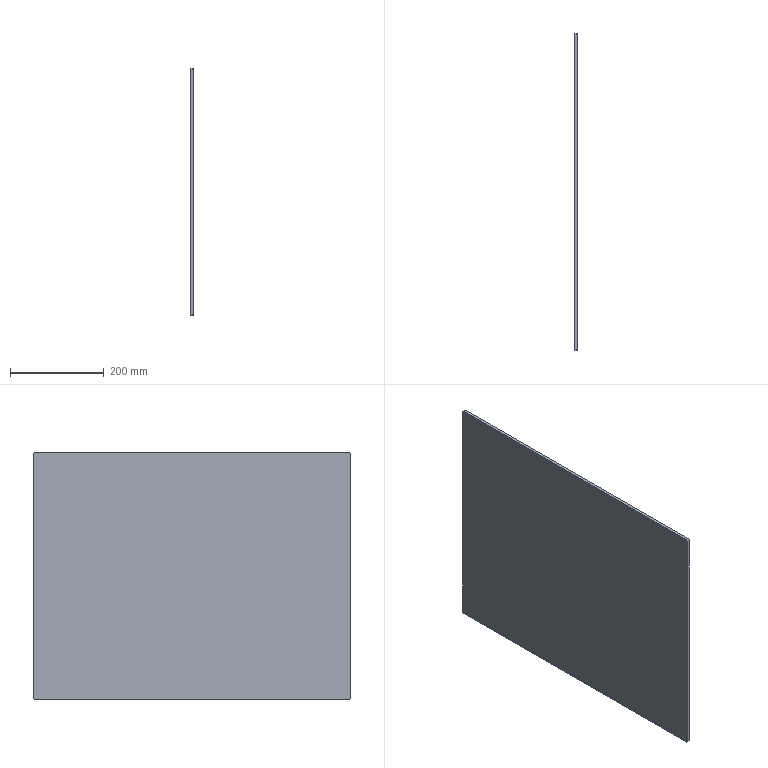Part | SolidWorks | features Chamfer 1, Extrusion 1 | 1 solid | 10 faces | box 6 x 677 x 528 mm | volume 2144688 mm3 | plane 10
STEP:
#1=CARTESIAN_POINT('',(3.,-336.5,-264.));
#2=VERTEX_POINT('',#1);
#3=CARTESIAN_POINT('',(3.,336.5,-264.));
#4=VERTEX_POINT('',#3);
#5=CARTESIAN_POINT('',(3.,338.5,-264.));
#6=DIRECTION('',(0.,1.,0.));
#7=VECTOR('',#6,1000.);
#8=LINE('',#5,#7);
#9=EDGE_CURVE('',#2,#4,#8,.T.);
#10=ORIENTED_EDGE('',*,*,#9,.F.);
#11=CARTESIAN_POINT('',(-3.,-336.5,-264.));
#12=VERTEX_POINT('',#11);
#13=CARTESIAN_POINT('',(3.,-336.5,-264.));
#14=DIRECTION('',(-1.,0.,0.));
#15=VECTOR('',#14,1000.);
#16=LINE('',#13,#15);
#17=EDGE_CURVE('',#2,#12,#16,.T.);
#18=ORIENTED_EDGE('',*,*,#17,.T.);
#19=CARTESIAN_POINT('',(-3.,336.5,-264.));
#20=VERTEX_POINT('',#19);
#21=CARTESIAN_POINT('',(-3.,338.5,-264.));
#22=DIRECTION('',(0.,1.,0.));
#23=VECTOR('',#22,1000.);
#24=LINE('',#21,#23);
#25=EDGE_CURVE('',#12,#20,#24,.T.);
#26=ORIENTED_EDGE('',*,*,#25,.T.);
#27=CARTESIAN_POINT('',(3.,336.5,-264.));
#28=DIRECTION('',(1.,0.,0.));
#29=VECTOR('',#28,1000.);
#30=LINE('',#27,#29);
#31=EDGE_CURVE('',#20,#4,#30,.T.);
#32=ORIENTED_EDGE('',*,*,#31,.T.);
#33=EDGE_LOOP('',(#10,#18,#26,#32));
#34=FACE_OUTER_BOUND('',#33,.T.);
#35=CARTESIAN_POINT('',(3.,338.5,-264.));
#36=DIRECTION('',(0.,0.,1.));
#37=DIRECTION('',(0.,-1.,0.));
#38=AXIS2_PLACEMENT_3D('',#35,#36,#37);
#39=PLANE('',#38);
#40=ADVANCED_FACE('',(#34),#39,.F.);
#41=CARTESIAN_POINT('',(3.,338.5,-262.));
#42=VERTEX_POINT('',#41);
#43=CARTESIAN_POINT('',(3.,338.5,262.));
#44=VERTEX_POINT('',#43);
#45=CARTESIAN_POINT('',(3.,338.5,264.));
#46=DIRECTION('',(0.,0.,1.));
#47=VECTOR('',#46,1000.);
#48=LINE('',#45,#47);
#49=EDGE_CURVE('',#42,#44,#48,.T.);
#50=ORIENTED_EDGE('',*,*,#49,.F.);
#51=CARTESIAN_POINT('',(-3.,338.5,-262.));
#52=VERTEX_POINT('',#51);
#53=CARTESIAN_POINT('',(3.,338.5,-262.));
#54=DIRECTION('',(-1.,0.,0.));
#55=VECTOR('',#54,1000.);
#56=LINE('',#53,#55);
#57=EDGE_CURVE('',#42,#52,#56,.T.);
#58=ORIENTED_EDGE('',*,*,#57,.T.);
#59=CARTESIAN_POINT('',(-3.,338.5,262.));
#60=VERTEX_POINT('',#59);
#61=CARTESIAN_POINT('',(-3.,338.5,264.));
#62=DIRECTION('',(0.,0.,1.));
#63=VECTOR('',#62,1000.);
#64=LINE('',#61,#63);
#65=EDGE_CURVE('',#52,#60,#64,.T.);
#66=ORIENTED_EDGE('',*,*,#65,.T.);
#67=CARTESIAN_POINT('',(3.,338.5,262.));
#68=DIRECTION('',(1.,0.,0.));
#69=VECTOR('',#68,1000.);
#70=LINE('',#67,#69);
#71=EDGE_CURVE('',#60,#44,#70,.T.);
#72=ORIENTED_EDGE('',*,*,#71,.T.);
#73=EDGE_LOOP('',(#50,#58,#66,#72));
#74=FACE_OUTER_BOUND('',#73,.T.);
#75=CARTESIAN_POINT('',(3.,338.5,264.));
#76=DIRECTION('',(0.,-1.,0.));
#77=DIRECTION('',(0.,0.,-1.));
#78=AXIS2_PLACEMENT_3D('',#75,#76,#77);
#79=PLANE('',#78);
#80=ADVANCED_FACE('',(#74),#79,.F.);
#81=CARTESIAN_POINT('',(-3.,336.5,264.));
#82=VERTEX_POINT('',#81);
#83=CARTESIAN_POINT('',(-3.,-336.5,264.));
#84=VERTEX_POINT('',#83);
#85=CARTESIAN_POINT('',(-3.,338.5,264.));
#86=DIRECTION('',(0.,-1.,0.));
#87=VECTOR('',#86,1000.);
#88=LINE('',#85,#87);
#89=EDGE_CURVE('',#82,#84,#88,.T.);
#90=ORIENTED_EDGE('',*,*,#89,.T.);
#91=CARTESIAN_POINT('',(3.,-336.5,264.));
#92=VERTEX_POINT('',#91);
#93=CARTESIAN_POINT('',(3.,-336.5,264.));
#94=DIRECTION('',(1.,0.,0.));
#95=VECTOR('',#94,1000.);
#96=LINE('',#93,#95);
#97=EDGE_CURVE('',#84,#92,#96,.T.);
#98=ORIENTED_EDGE('',*,*,#97,.T.);
#99=CARTESIAN_POINT('',(3.,336.5,264.));
#100=VERTEX_POINT('',#99);
#101=CARTESIAN_POINT('',(3.,338.5,264.));
#102=DIRECTION('',(0.,-1.,0.));
#103=VECTOR('',#102,1000.);
#104=LINE('',#101,#103);
#105=EDGE_CURVE('',#100,#92,#104,.T.);
#106=ORIENTED_EDGE('',*,*,#105,.F.);
#107=CARTESIAN_POINT('',(3.,336.5,264.));
#108=DIRECTION('',(-1.,0.,0.));
#109=VECTOR('',#108,1000.);
#110=LINE('',#107,#109);
#111=EDGE_CURVE('',#100,#82,#110,.T.);
#112=ORIENTED_EDGE('',*,*,#111,.T.);
#113=EDGE_LOOP('',(#90,#98,#106,#112));
#114=FACE_OUTER_BOUND('',#113,.T.);
#115=CARTESIAN_POINT('',(3.,338.5,264.));
#116=DIRECTION('',(0.,0.,-1.));
#117=DIRECTION('',(0.,1.,0.));
#118=AXIS2_PLACEMENT_3D('',#115,#116,#117);
#119=PLANE('',#118);
#120=ADVANCED_FACE('',(#114),#119,.F.);
#121=CARTESIAN_POINT('',(3.,-338.5,262.));
#122=VERTEX_POINT('',#121);
#123=CARTESIAN_POINT('',(3.,-338.5,-262.));
#124=VERTEX_POINT('',#123);
#125=CARTESIAN_POINT('',(3.,-338.5,264.));
#126=DIRECTION('',(0.,0.,-1.));
#127=VECTOR('',#126,1000.);
#128=LINE('',#125,#127);
#129=EDGE_CURVE('',#122,#124,#128,.T.);
#130=ORIENTED_EDGE('',*,*,#129,.F.);
#131=CARTESIAN_POINT('',(-3.,-338.5,262.));
#132=VERTEX_POINT('',#131);
#133=CARTESIAN_POINT('',(3.,-338.5,262.));
#134=DIRECTION('',(-1.,0.,0.));
#135=VECTOR('',#134,1000.);
#136=LINE('',#133,#135);
#137=EDGE_CURVE('',#122,#132,#136,.T.);
#138=ORIENTED_EDGE('',*,*,#137,.T.);
#139=CARTESIAN_POINT('',(-3.,-338.5,-262.));
#140=VERTEX_POINT('',#139);
#141=CARTESIAN_POINT('',(-3.,-338.5,264.));
#142=DIRECTION('',(0.,0.,-1.));
#143=VECTOR('',#142,1000.);
#144=LINE('',#141,#143);
#145=EDGE_CURVE('',#132,#140,#144,.T.);
#146=ORIENTED_EDGE('',*,*,#145,.T.);
#147=CARTESIAN_POINT('',(3.,-338.5,-262.));
#148=DIRECTION('',(1.,0.,0.));
#149=VECTOR('',#148,1000.);
#150=LINE('',#147,#149);
#151=EDGE_CURVE('',#140,#124,#150,.T.);
#152=ORIENTED_EDGE('',*,*,#151,.T.);
#153=EDGE_LOOP('',(#130,#138,#146,#152));
#154=FACE_OUTER_BOUND('',#153,.T.);
#155=CARTESIAN_POINT('',(3.,-338.5,264.));
#156=DIRECTION('',(0.,1.,0.));
#157=DIRECTION('',(0.,0.,1.));
#158=AXIS2_PLACEMENT_3D('',#155,#156,#157);
#159=PLANE('',#158);
#160=ADVANCED_FACE('',(#154),#159,.F.);
#161=ORIENTED_EDGE('',*,*,#105,.T.);
#162=CARTESIAN_POINT('',(3.,-300.25,300.25));
#163=DIRECTION('',(0.,-0.7071,-0.7071));
#164=VECTOR('',#163,1000.);
#165=LINE('',#162,#164);
#166=EDGE_CURVE('',#92,#122,#165,.T.);
#167=ORIENTED_EDGE('',*,*,#166,.T.);
#168=ORIENTED_EDGE('',*,*,#129,.T.);
#169=CARTESIAN_POINT('',(3.,-300.25,-300.25));
#170=DIRECTION('',(0.,0.7071,-0.7071));
#171=VECTOR('',#170,1000.);
#172=LINE('',#169,#171);
#173=EDGE_CURVE('',#124,#2,#172,.T.);
#174=ORIENTED_EDGE('',*,*,#173,.T.);
#175=ORIENTED_EDGE('',*,*,#9,.T.);
#176=CARTESIAN_POINT('',(3.,300.25,-300.25));
#177=DIRECTION('',(0.,0.7071,0.7071));
#178=VECTOR('',#177,1000.);
#179=LINE('',#176,#178);
#180=EDGE_CURVE('',#4,#42,#179,.T.);
#181=ORIENTED_EDGE('',*,*,#180,.T.);
#182=ORIENTED_EDGE('',*,*,#49,.T.);
#183=CARTESIAN_POINT('',(3.,300.25,300.25));
#184=DIRECTION('',(0.,-0.7071,0.7071));
#185=VECTOR('',#184,1000.);
#186=LINE('',#183,#185);
#187=EDGE_CURVE('',#44,#100,#186,.T.);
#188=ORIENTED_EDGE('',*,*,#187,.T.);
#189=EDGE_LOOP('',(#161,#167,#168,#174,#175,#181,#182,#188));
#190=FACE_OUTER_BOUND('',#189,.T.);
#191=CARTESIAN_POINT('',(3.,0.,0.));
#192=DIRECTION('',(1.,0.,0.));
#193=DIRECTION('',(0.,0.,-1.));
#194=AXIS2_PLACEMENT_3D('',#191,#192,#193);
#195=PLANE('',#194);
#196=ADVANCED_FACE('',(#190),#195,.T.);
#197=ORIENTED_EDGE('',*,*,#145,.F.);
#198=CARTESIAN_POINT('',(-3.,-338.5,262.));
#199=DIRECTION('',(0.,0.7071,0.7071));
#200=VECTOR('',#199,1000.);
#201=LINE('',#198,#200);
#202=EDGE_CURVE('',#132,#84,#201,.T.);
#203=ORIENTED_EDGE('',*,*,#202,.T.);
#204=ORIENTED_EDGE('',*,*,#89,.F.);
#205=CARTESIAN_POINT('',(-3.,336.5,264.));
#206=DIRECTION('',(0.,0.7071,-0.7071));
#207=VECTOR('',#206,1000.);
#208=LINE('',#205,#207);
#209=EDGE_CURVE('',#82,#60,#208,.T.);
#210=ORIENTED_EDGE('',*,*,#209,.T.);
#211=ORIENTED_EDGE('',*,*,#65,.F.);
#212=CARTESIAN_POINT('',(-3.,338.5,-262.));
#213=DIRECTION('',(0.,-0.7071,-0.7071));
#214=VECTOR('',#213,1000.);
#215=LINE('',#212,#214);
#216=EDGE_CURVE('',#52,#20,#215,.T.);
#217=ORIENTED_EDGE('',*,*,#216,.T.);
#218=ORIENTED_EDGE('',*,*,#25,.F.);
#219=CARTESIAN_POINT('',(-3.,-336.5,-264.));
#220=DIRECTION('',(0.,-0.7071,0.7071));
#221=VECTOR('',#220,1000.);
#222=LINE('',#219,#221);
#223=EDGE_CURVE('',#12,#140,#222,.T.);
#224=ORIENTED_EDGE('',*,*,#223,.T.);
#225=EDGE_LOOP('',(#197,#203,#204,#210,#211,#217,#218,#224));
#226=FACE_OUTER_BOUND('',#225,.T.);
#227=CARTESIAN_POINT('',(-3.,0.,0.));
#228=DIRECTION('',(1.,0.,0.));
#229=DIRECTION('',(0.,0.,-1.));
#230=AXIS2_PLACEMENT_3D('',#227,#228,#229);
#231=PLANE('',#230);
#232=ADVANCED_FACE('',(#226),#231,.F.);
#233=ORIENTED_EDGE('',*,*,#166,.F.);
#234=ORIENTED_EDGE('',*,*,#97,.F.);
#235=ORIENTED_EDGE('',*,*,#202,.F.);
#236=ORIENTED_EDGE('',*,*,#137,.F.);
#237=EDGE_LOOP('',(#233,#234,#235,#236));
#238=FACE_OUTER_BOUND('',#237,.T.);
#239=CARTESIAN_POINT('',(3.,-338.5,262.));
#240=DIRECTION('',(0.,0.7071,-0.7071));
#241=DIRECTION('',(-1.,0.,0.));
#242=AXIS2_PLACEMENT_3D('',#239,#240,#241);
#243=PLANE('',#242);
#244=ADVANCED_FACE('',(#238),#243,.F.);
#245=ORIENTED_EDGE('',*,*,#173,.F.);
#246=ORIENTED_EDGE('',*,*,#151,.F.);
#247=ORIENTED_EDGE('',*,*,#223,.F.);
#248=ORIENTED_EDGE('',*,*,#17,.F.);
#249=EDGE_LOOP('',(#245,#246,#247,#248));
#250=FACE_OUTER_BOUND('',#249,.T.);
#251=CARTESIAN_POINT('',(3.,-336.5,-264.));
#252=DIRECTION('',(0.,0.7071,0.7071));
#253=DIRECTION('',(-1.,0.,0.));
#254=AXIS2_PLACEMENT_3D('',#251,#252,#253);
#255=PLANE('',#254);
#256=ADVANCED_FACE('',(#250),#255,.F.);
#257=ORIENTED_EDGE('',*,*,#180,.F.);
#258=ORIENTED_EDGE('',*,*,#31,.F.);
#259=ORIENTED_EDGE('',*,*,#216,.F.);
#260=ORIENTED_EDGE('',*,*,#57,.F.);
#261=EDGE_LOOP('',(#257,#258,#259,#260));
#262=FACE_OUTER_BOUND('',#261,.T.);
#263=CARTESIAN_POINT('',(3.,338.5,-262.));
#264=DIRECTION('',(0.,-0.7071,0.7071));
#265=DIRECTION('',(-1.,0.,0.));
#266=AXIS2_PLACEMENT_3D('',#263,#264,#265);
#267=PLANE('',#266);
#268=ADVANCED_FACE('',(#262),#267,.F.);
#269=ORIENTED_EDGE('',*,*,#187,.F.);
#270=ORIENTED_EDGE('',*,*,#71,.F.);
#271=ORIENTED_EDGE('',*,*,#209,.F.);
#272=ORIENTED_EDGE('',*,*,#111,.F.);
#273=EDGE_LOOP('',(#269,#270,#271,#272));
#274=FACE_OUTER_BOUND('',#273,.T.);
#275=CARTESIAN_POINT('',(3.,336.5,264.));
#276=DIRECTION('',(0.,-0.7071,-0.7071));
#277=DIRECTION('',(-1.,0.,0.));
#278=AXIS2_PLACEMENT_3D('',#275,#276,#277);
#279=PLANE('',#278);
#280=ADVANCED_FACE('',(#274),#279,.F.);
#281=CLOSED_SHELL('',(#40,#80,#120,#160,#196,#232,#244,#256,#268,#280));
#282=MANIFOLD_SOLID_BREP('',#281);
#283=CARTESIAN_POINT('',(0.,0.,0.));
#284=DIRECTION('',(0.,0.,1.));
#285=DIRECTION('',(1.,0.,0.));
#286=AXIS2_PLACEMENT_3D('',#283,#284,#285);
#287=(LENGTH_UNIT()NAMED_UNIT(*)SI_UNIT(.MILLI.,.METRE.));
#288=UNCERTAINTY_MEASURE_WITH_UNIT(LENGTH_MEASURE(0.00001),#287,'','');
#289=(NAMED_UNIT(*)PLANE_ANGLE_UNIT()SI_UNIT($,.RADIAN.));
#290=(NAMED_UNIT(*)SI_UNIT($,.STERADIAN.)SOLID_ANGLE_UNIT());
#291=(GEOMETRIC_REPRESENTATION_CONTEXT(3)GLOBAL_UNCERTAINTY_ASSIGNED_CONTEXT((#288))GLOBAL_UNIT_ASSIGNED_CONTEXT((#287,#289,#290))REPRESENTATION_CONTEXT('',''));
#292=ADVANCED_BREP_SHAPE_REPRESENTATION('',(#282,#286),#291);